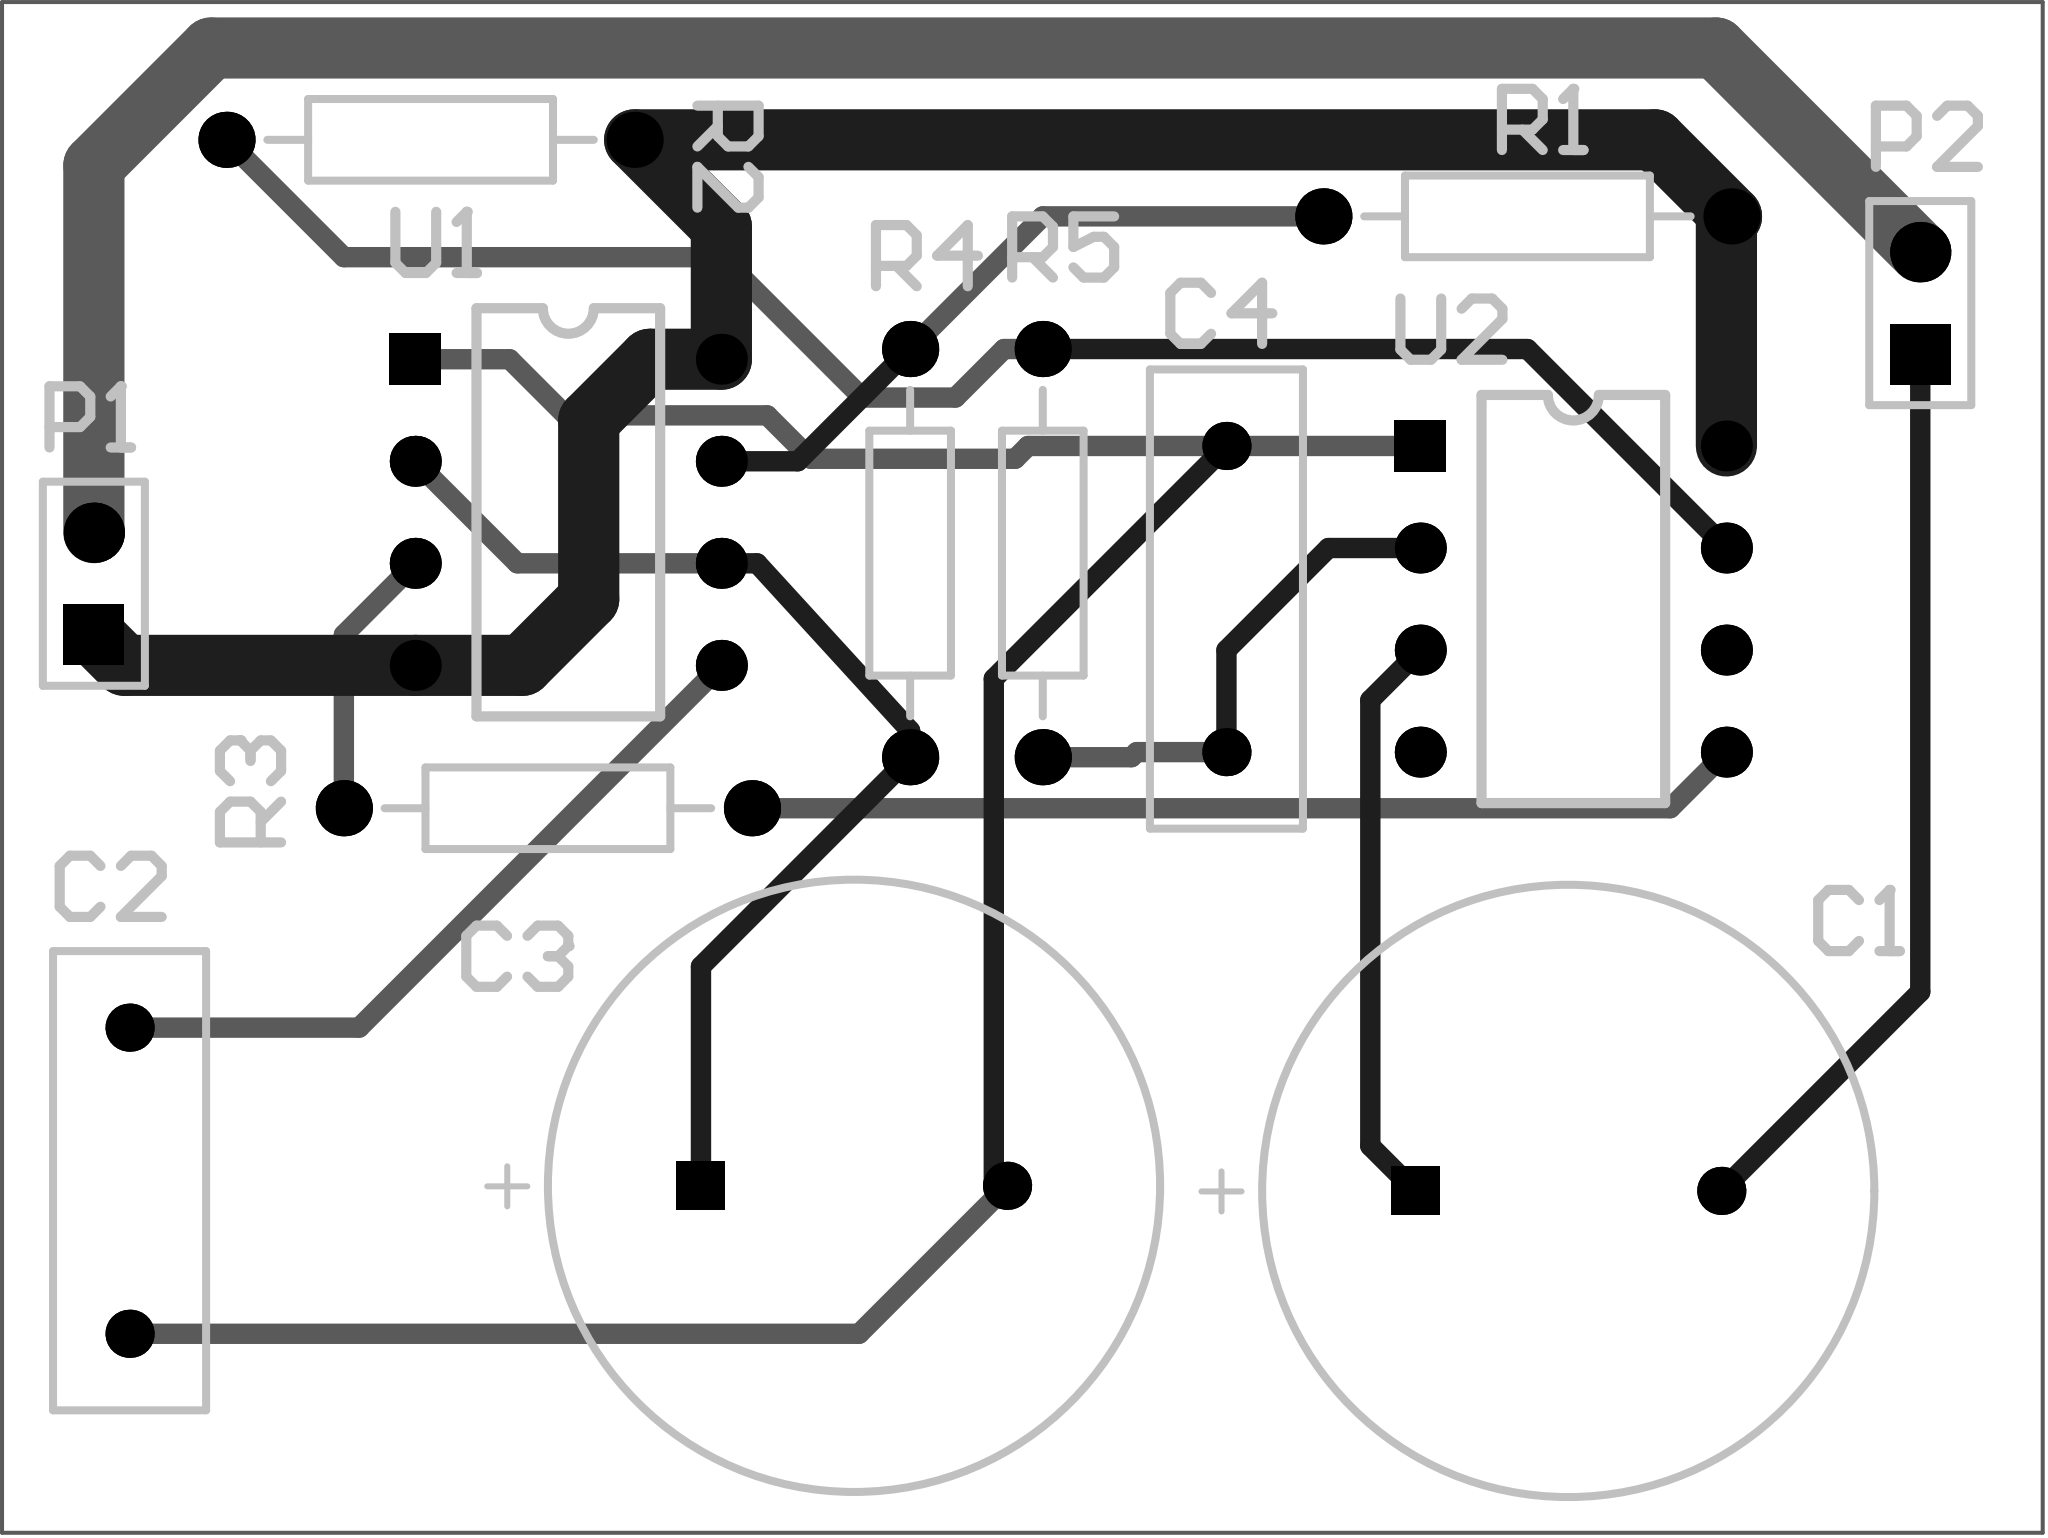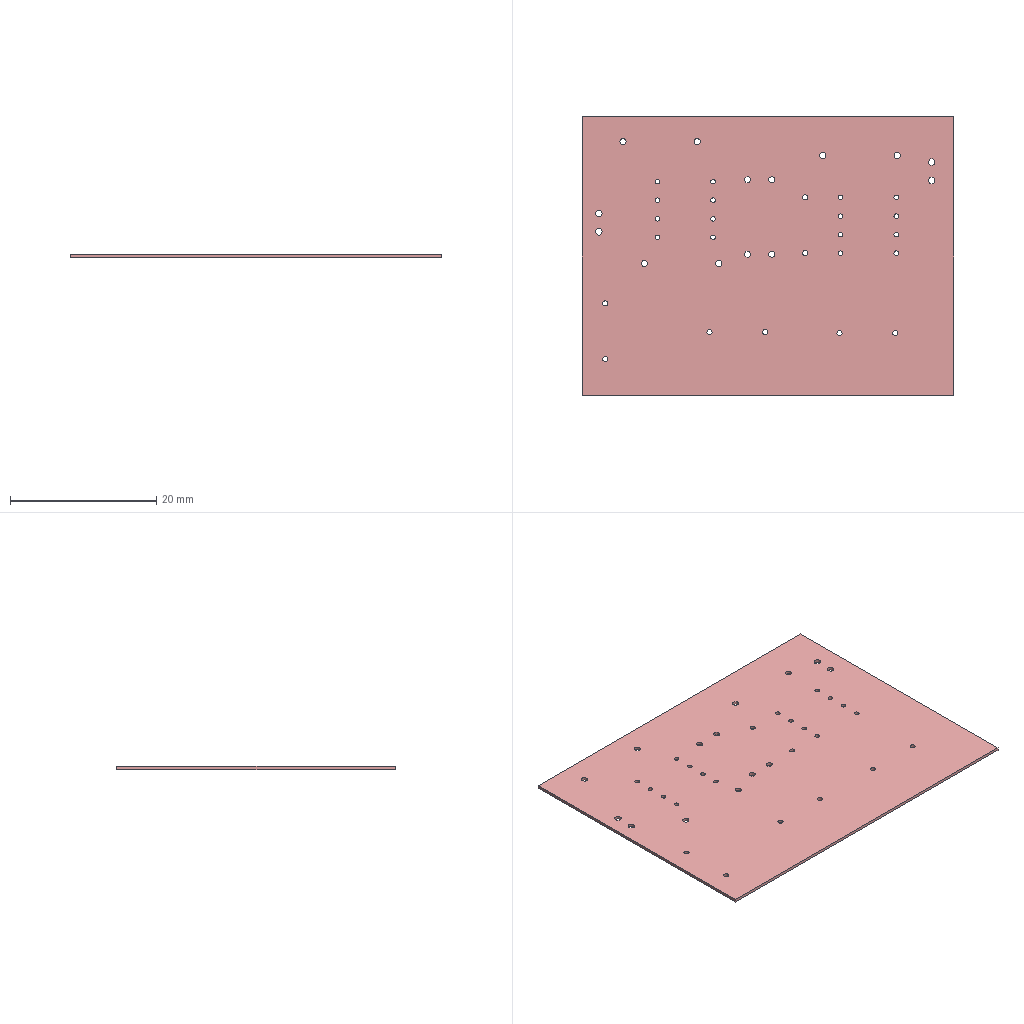Circuit board layout | Altium Designer | box 50.8 x 38.1 x 0.4 mm
Layer stack:
# Altium Designer layer stack of  (unit mm; dielectric type: 0 none, 1 core, 2 prepreg, 3 surface material)
index,name,kind,layer,copper_thickness_mm,dielectric_type,dielectric_thickness_mm,dielectric_material,dielectric_constant
0,Top Paste,other,,,,,,
1,Top Overlay,other,,,,,,
2,Top Solder,dielectric,,,3,0.0102,Solder Resist,3.5
3,Top Layer,copper,Top Layer,0.0356,,,,
4,Dielectric 1,dielectric,,,0,0.32,FR-4,4.8
5,Bottom Layer,copper,Bottom Layer,0.0356,,,,
6,Bottom Solder,dielectric,,,3,0.0102,Solder Resist,3.5
7,Bottom Overlay,other,,,,,,
8,Bottom Paste,other,,,,,,
# drill layer pairs: low layer,high layer
drill_pair,Top Layer,Bottom Layer
Part placement:
Designator,Comment,Layer,Footprint,Center-X(mm),Center-Y(mm),Rotation
U2,NE555,TopLayer,DIP8,64.516,48.641,0
U1,NE555,TopLayer,DIP8,39.497,50.8,0
R5,Res2,TopLayer,AXIAL-0.4,51.308,49.784,270
R4,Res2,TopLayer,AXIAL-0.4,48.006,49.784,90
R3,Res2,TopLayer,AXIAL-0.4,38.989,43.434,180
R2,Res2,TopLayer,AXIAL-0.4,36.068,60.071,360
R1,Res2,TopLayer,AXIAL-0.4,63.373,58.166,360
P2,Header 2,TopLayer,HDR1X2,73.152,56.007,90
P1,Header 2,TopLayer,HDR1X2,27.686,49.022,90
C4,Cap,TopLayer,RAD-0.3,55.88,48.641,270
C3,Cap Pol1,TopLayer,RB7.6-15,46.609,34.036,180
C2,Cap,TopLayer,RAD-0.3,28.575,34.163,90
C1,Cap Pol1,TopLayer,RB7.6-15,64.389,33.909,180
Pad and via stacks:
# Altium Designer via and pad stacks of  (unit mm). Each distinct definition once, with the count of objects using it.
# via: kind,start_layer,end_layer,hole_mm,diameter_mm,mode(0 simple;1 top-mid-bottom;2 full stack),diameter_per_layer,count,example_net
# pad: kind,layer,hole_mm,hole_type(0 round;1 square;2 slot),plating,top_size,top_shape(1 round;2 rect;3 octagon;9 rounded rect),mid_size,bottom_size,mode,footprint,size_per_layer,count,example
pad,Multi-Layer,0.85,0,plated,1.4x1.4,1,1.4x1.4,1.4x1.4,0,AXIAL-0.4,,10,R2.1
pad,Multi-Layer,0.635,0,plated,1.27x1.27,1,1.27x1.27,1.27x1.27,0,DIP8,,14,U2.5
pad,Multi-Layer,0.635,0,plated,1.27x1.27,2,1.27x1.27,1.27x1.27,0,DIP8,,2,U2.1
pad,Multi-Layer,0.7,0,plated,1.2x1.2,2,1.2x1.2,1.2x1.2,0,RB7.6-15,,2,C1.1
pad,Multi-Layer,0.7,0,plated,1.2x1.2,1,1.2x1.2,1.2x1.2,0,RB7.6-15,,2,C1.2
pad,Multi-Layer,0.7,0,plated,1.2x1.2,1,1.2x1.2,1.2x1.2,0,RAD-0.3,,4,C2.2
pad,Multi-Layer,0.9,0,plated,1.5x1.5,2,1.5x1.5,1.5x1.5,0,HDR1X2,,2,P2.1
pad,Multi-Layer,0.9,0,plated,1.5x1.5,1,1.5x1.5,1.5x1.5,0,HDR1X2,,2,P2.2
Design rules, without the lines most boards share:
# Altium Designer design rules of  (exported by Altium Designer, unit mm)
# columns: name | kind | enabled | priority | scope1 | scope2 | descriptor | typed fields (field=value)
Width | 2 | enabled | 1 | All | All | Width Constraint (Min=20mil) (Max=60mil) (Preferred=20mil) (All) |
GND | 2 | enabled | 2 | InNet('GND') | All | Width Constraint (Min=60mil) (Max=60mil) (Preferred=60mil) (InNet('GND')) |
HoleToHoleClearance | 52 | enabled | 1 | All | All | Hole To Hole Clearance (Gap=10mil) (All),(All) | gap=0.254
DiffPairsRouting | 51 | enabled | 1 | All | All | Differential Pairs Uncoupled Length using the Gap Constraints (Min=10mil) (Max=10mil) (Prefered=10mil)  and Width Constraints (Min=15mil) (Max=15mil) (Prefered=15mil) (All) |
SolderMaskExpansion | 13 | enabled | 1 | All | All | Solder Mask Expansion (Expansion =4mil) (All) | expansion=0.1016
PasteMaskExpansion | 14 | enabled | 1 | All | All | Paste Mask Expansion (Expansion =0mil) (All) | expansion=0
RoutingVias | 11 | enabled | 1 | All | All | Routing Via (MinHoleWidth=28mil) (MaxHoleWidth=28mil) (PreferredHoleWidth=28mil) (MinWidth=50mil) (MaxWidth=50mil) (PreferedWidth=50mil) (All) | via_min_hole=0.7112 via_max_hole=0.7112 via_preferred_diameter=1.27 via_preferred_hole=0.7112
VCC | 2 | enabled | 3 | InNet('VCC') | All | Width Constraint (Min=60mil) (Max=60mil) (Preferred=60mil) (InNet('VCC')) |
PolygonConnect | 20 | enabled | 1 | All | All | Polygon Connect Rule(Relief Connect )(Conductor Width=10mil) (Relief Angle=90 Angle) (Entries=4) (Air Gap Width=10mil) (All),(All) | connect_style(0=relief,1=direct,2=none)=0 relief_conductor_width=0.254 relief_entries=4
PlaneConnect | 6 | enabled | 1 | All | All | Power Plane Connect Rule(Relief Connect )(Expansion=20mil) (Conductor Width=10mil) (Air Gap=10mil) (Entries=4) (All) | relief_conductor_width=0.254 relief_entries=4 relief_expansion=0.508
Clearance | 0 | enabled | 1 | All | All | Clearance Constraint (Gap=10mil) (All),(All) | gap=0.254